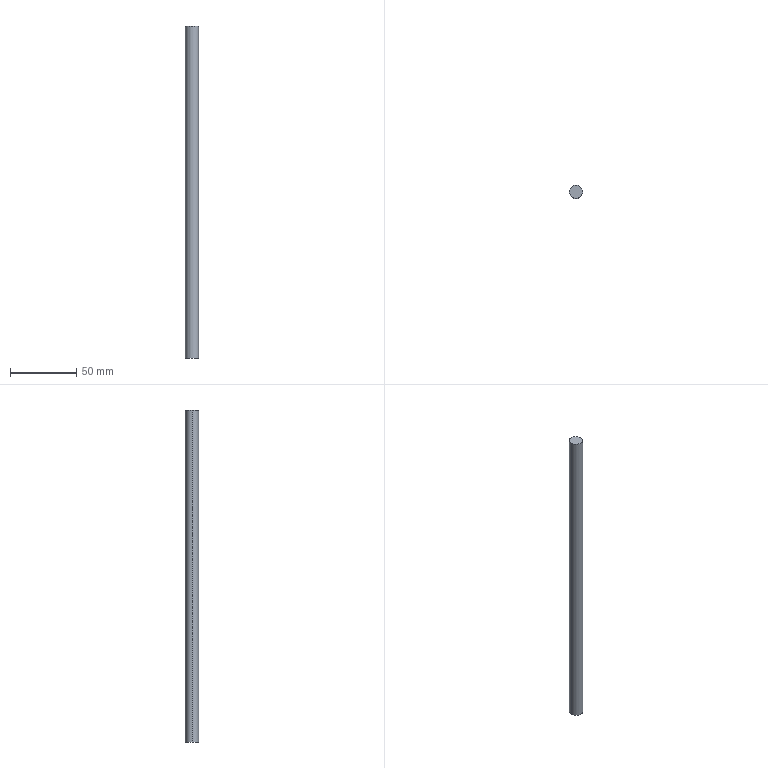Part | SolidWorks | features Extrusion 1 | 1 solid | 4 faces | box 10 x 10 x 250 mm | volume 19635 mm3 | cylinder 2 | plane 2 | commonest cylinder face diameters 10 x2
STEP:
#1=CARTESIAN_POINT('',(5.,0.,250.));
#2=VERTEX_POINT('',#1);
#3=CARTESIAN_POINT('',(-5.,0.,250.));
#4=VERTEX_POINT('',#3);
#5=CARTESIAN_POINT('',(0.,0.,250.));
#6=DIRECTION('',(0.,0.,1.));
#7=DIRECTION('',(1.,0.,0.));
#8=AXIS2_PLACEMENT_3D('',#5,#6,#7);
#9=CIRCLE('',#8,5.);
#10=EDGE_CURVE('',#2,#4,#9,.T.);
#11=ORIENTED_EDGE('',*,*,#10,.F.);
#12=CARTESIAN_POINT('',(5.,0.,0.));
#13=VERTEX_POINT('',#12);
#14=CARTESIAN_POINT('',(5.,0.,250.));
#15=DIRECTION('',(0.,0.,-1.));
#16=VECTOR('',#15,1000.);
#17=LINE('',#14,#16);
#18=EDGE_CURVE('',#2,#13,#17,.T.);
#19=ORIENTED_EDGE('',*,*,#18,.T.);
#20=CARTESIAN_POINT('',(-5.,0.,0.));
#21=VERTEX_POINT('',#20);
#22=CARTESIAN_POINT('',(0.,0.,0.));
#23=DIRECTION('',(0.,0.,1.));
#24=DIRECTION('',(1.,0.,0.));
#25=AXIS2_PLACEMENT_3D('',#22,#23,#24);
#26=CIRCLE('',#25,5.);
#27=EDGE_CURVE('',#13,#21,#26,.T.);
#28=ORIENTED_EDGE('',*,*,#27,.T.);
#29=CARTESIAN_POINT('',(-5.,0.,250.));
#30=DIRECTION('',(0.,0.,-1.));
#31=VECTOR('',#30,1000.);
#32=LINE('',#29,#31);
#33=EDGE_CURVE('',#4,#21,#32,.T.);
#34=ORIENTED_EDGE('',*,*,#33,.F.);
#35=EDGE_LOOP('',(#11,#19,#28,#34));
#36=FACE_OUTER_BOUND('',#35,.T.);
#37=CARTESIAN_POINT('',(0.,0.,250.));
#38=DIRECTION('',(0.,0.,-1.));
#39=DIRECTION('',(-1.,0.,0.));
#40=AXIS2_PLACEMENT_3D('',#37,#38,#39);
#41=CYLINDRICAL_SURFACE('',#40,5.);
#42=ADVANCED_FACE('',(#36),#41,.T.);
#43=ORIENTED_EDGE('',*,*,#18,.F.);
#44=CARTESIAN_POINT('',(0.,0.,250.));
#45=DIRECTION('',(0.,0.,1.));
#46=DIRECTION('',(1.,0.,0.));
#47=AXIS2_PLACEMENT_3D('',#44,#45,#46);
#48=CIRCLE('',#47,5.);
#49=EDGE_CURVE('',#4,#2,#48,.T.);
#50=ORIENTED_EDGE('',*,*,#49,.F.);
#51=ORIENTED_EDGE('',*,*,#33,.T.);
#52=CARTESIAN_POINT('',(0.,0.,0.));
#53=DIRECTION('',(0.,0.,1.));
#54=DIRECTION('',(1.,0.,0.));
#55=AXIS2_PLACEMENT_3D('',#52,#53,#54);
#56=CIRCLE('',#55,5.);
#57=EDGE_CURVE('',#21,#13,#56,.T.);
#58=ORIENTED_EDGE('',*,*,#57,.T.);
#59=EDGE_LOOP('',(#43,#50,#51,#58));
#60=FACE_OUTER_BOUND('',#59,.T.);
#61=CARTESIAN_POINT('',(0.,0.,250.));
#62=DIRECTION('',(0.,0.,-1.));
#63=DIRECTION('',(-1.,0.,0.));
#64=AXIS2_PLACEMENT_3D('',#61,#62,#63);
#65=CYLINDRICAL_SURFACE('',#64,5.);
#66=ADVANCED_FACE('',(#60),#65,.T.);
#67=ORIENTED_EDGE('',*,*,#49,.T.);
#68=ORIENTED_EDGE('',*,*,#10,.T.);
#69=EDGE_LOOP('',(#67,#68));
#70=FACE_OUTER_BOUND('',#69,.T.);
#71=CARTESIAN_POINT('',(0.,0.,250.));
#72=DIRECTION('',(0.,0.,1.));
#73=DIRECTION('',(1.,0.,0.));
#74=AXIS2_PLACEMENT_3D('',#71,#72,#73);
#75=PLANE('',#74);
#76=ADVANCED_FACE('',(#70),#75,.T.);
#77=ORIENTED_EDGE('',*,*,#57,.F.);
#78=ORIENTED_EDGE('',*,*,#27,.F.);
#79=EDGE_LOOP('',(#77,#78));
#80=FACE_OUTER_BOUND('',#79,.T.);
#81=CARTESIAN_POINT('',(0.,0.,0.));
#82=DIRECTION('',(0.,0.,1.));
#83=DIRECTION('',(1.,0.,0.));
#84=AXIS2_PLACEMENT_3D('',#81,#82,#83);
#85=PLANE('',#84);
#86=ADVANCED_FACE('',(#80),#85,.F.);
#87=CLOSED_SHELL('',(#42,#66,#76,#86));
#88=MANIFOLD_SOLID_BREP('',#87);
#89=CARTESIAN_POINT('',(0.,0.,0.));
#90=DIRECTION('',(0.,0.,1.));
#91=DIRECTION('',(1.,0.,0.));
#92=AXIS2_PLACEMENT_3D('',#89,#90,#91);
#93=(LENGTH_UNIT()NAMED_UNIT(*)SI_UNIT(.MILLI.,.METRE.));
#94=UNCERTAINTY_MEASURE_WITH_UNIT(LENGTH_MEASURE(0.00001),#93,'','');
#95=(NAMED_UNIT(*)PLANE_ANGLE_UNIT()SI_UNIT($,.RADIAN.));
#96=(NAMED_UNIT(*)SI_UNIT($,.STERADIAN.)SOLID_ANGLE_UNIT());
#97=(GEOMETRIC_REPRESENTATION_CONTEXT(3)GLOBAL_UNCERTAINTY_ASSIGNED_CONTEXT((#94))GLOBAL_UNIT_ASSIGNED_CONTEXT((#93,#95,#96))REPRESENTATION_CONTEXT('',''));
#98=ADVANCED_BREP_SHAPE_REPRESENTATION('',(#88,#92),#97);